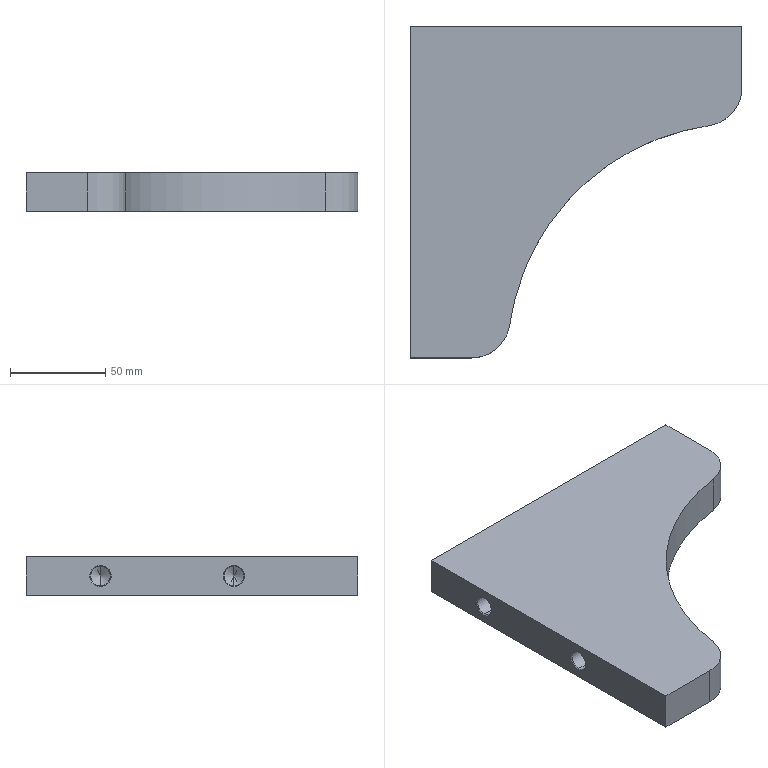Part | STEP file | Chain press plate | 1 solid | 21 faces | box 174 x 174 x 20 mm | volume 359243 mm3 | cone 8 | cylinder 7 | plane 6 | commonest cylinder face diameters 10.2 x4 40 x2 246 x1
STEP:
#1=CARTESIAN_POINT('',(0.,0.,0.));
#2=DIRECTION('',(0.,0.,1.));
#3=DIRECTION('',(1.,0.,0.));
#4=AXIS2_PLACEMENT_3D('',#1,#2,#3);
#5=CARTESIAN_POINT('',(0.5,-39.,15.1));
#6=VERTEX_POINT('',#5);
#7=CARTESIAN_POINT('',(0.,-39.,15.6));
#8=VERTEX_POINT('',#7);
#9=CARTESIAN_POINT('',(0.5,-39.,15.1));
#10=DIRECTION('',(-0.7071,0.,0.7071));
#11=VECTOR('',#10,1.);
#12=LINE('',#9,#11);
#13=CARTESIAN_POINT('',(0.5,-39.,10.));
#14=DIRECTION('',(-1.,0.,0.));
#15=DIRECTION('',(0.,0.,1.));
#16=AXIS2_PLACEMENT_3D('',#13,#14,#15);
#17=CONICAL_SURFACE('',#16,5.1,0.7854);
#18=CARTESIAN_POINT('',(6.283,0.));
#19=DIRECTION('',(0.,1.));
#20=VECTOR('',#19,1.);
#21=LINE('',#18,#20);
#22=(GEOMETRIC_REPRESENTATION_CONTEXT(2)PARAMETRIC_REPRESENTATION_CONTEXT()REPRESENTATION_CONTEXT('',''));
#23=DEFINITIONAL_REPRESENTATION('',(#21),#22);
#24=PCURVE('',#17,#23);
#25=CARTESIAN_POINT('',(0.5,-39.,10.));
#26=DIRECTION('',(-1.,0.,0.));
#27=DIRECTION('',(0.,0.,1.));
#28=AXIS2_PLACEMENT_3D('',#25,#26,#27);
#29=CONICAL_SURFACE('',#28,5.1,0.7854);
#30=CARTESIAN_POINT('',(0.,0.));
#31=DIRECTION('',(0.,1.));
#32=VECTOR('',#31,1.);
#33=LINE('',#30,#32);
#34=(GEOMETRIC_REPRESENTATION_CONTEXT(2)PARAMETRIC_REPRESENTATION_CONTEXT()REPRESENTATION_CONTEXT('',''));
#35=DEFINITIONAL_REPRESENTATION('',(#33),#34);
#36=PCURVE('',#29,#35);
#37=SURFACE_CURVE('',#12,(#24,#36),.PCURVE_S1.);
#38=EDGE_CURVE('',#6,#8,#37,.T.);
#39=ORIENTED_EDGE('',*,*,#38,.T.);
#40=CARTESIAN_POINT('',(0.,-39.,4.4));
#41=VERTEX_POINT('',#40);
#42=CARTESIAN_POINT('',(0.,-39.,10.));
#43=DIRECTION('',(1.,0.,0.));
#44=DIRECTION('',(0.,1.,0.));
#45=AXIS2_PLACEMENT_3D('',#42,#43,#44);
#46=CIRCLE('',#45,5.6);
#47=CARTESIAN_POINT('',(7.854,0.5));
#48=DIRECTION('',(-1.,0.));
#49=VECTOR('',#48,1.);
#50=LINE('',#47,#49);
#51=(GEOMETRIC_REPRESENTATION_CONTEXT(2)PARAMETRIC_REPRESENTATION_CONTEXT()REPRESENTATION_CONTEXT('',''));
#52=DEFINITIONAL_REPRESENTATION('',(#50),#51);
#53=PCURVE('',#17,#52);
#54=CARTESIAN_POINT('',(0.,0.,20.));
#55=DIRECTION('',(1.,0.,0.));
#56=DIRECTION('',(0.,1.,0.));
#57=AXIS2_PLACEMENT_3D('',#54,#55,#56);
#58=PLANE('',#57);
#59=CARTESIAN_POINT('',(-39.,-10.));
#60=DIRECTION('',(1.,0.));
#61=AXIS2_PLACEMENT_2D('',#59,#60);
#62=CIRCLE('',#61,5.6);
#63=(GEOMETRIC_REPRESENTATION_CONTEXT(2)PARAMETRIC_REPRESENTATION_CONTEXT()REPRESENTATION_CONTEXT('',''));
#64=DEFINITIONAL_REPRESENTATION('',(#62),#63);
#65=PCURVE('',#58,#64);
#66=SURFACE_CURVE('',#46,(#53,#65),.PCURVE_S1.);
#67=EDGE_CURVE('',#8,#41,#66,.T.);
#68=ORIENTED_EDGE('',*,*,#67,.T.);
#69=CARTESIAN_POINT('',(0.5,-39.,4.9));
#70=VERTEX_POINT('',#69);
#71=CARTESIAN_POINT('',(0.5,-39.,4.9));
#72=DIRECTION('',(-0.7071,0.,-0.7071));
#73=VECTOR('',#72,1.);
#74=LINE('',#71,#73);
#75=CARTESIAN_POINT('',(3.142,0.));
#76=DIRECTION('',(0.,1.));
#77=VECTOR('',#76,1.);
#78=LINE('',#75,#77);
#79=(GEOMETRIC_REPRESENTATION_CONTEXT(2)PARAMETRIC_REPRESENTATION_CONTEXT()REPRESENTATION_CONTEXT('',''));
#80=DEFINITIONAL_REPRESENTATION('',(#78),#79);
#81=PCURVE('',#17,#80);
#82=CARTESIAN_POINT('',(3.142,0.));
#83=DIRECTION('',(0.,1.));
#84=VECTOR('',#83,1.);
#85=LINE('',#82,#84);
#86=(GEOMETRIC_REPRESENTATION_CONTEXT(2)PARAMETRIC_REPRESENTATION_CONTEXT()REPRESENTATION_CONTEXT('',''));
#87=DEFINITIONAL_REPRESENTATION('',(#85),#86);
#88=PCURVE('',#29,#87);
#89=SURFACE_CURVE('',#74,(#81,#88),.PCURVE_S1.);
#90=EDGE_CURVE('',#70,#41,#89,.T.);
#91=ORIENTED_EDGE('',*,*,#90,.F.);
#92=CARTESIAN_POINT('',(0.5,-39.,10.));
#93=DIRECTION('',(-1.,0.,0.));
#94=DIRECTION('',(0.,0.,-1.));
#95=AXIS2_PLACEMENT_3D('',#92,#93,#94);
#96=CIRCLE('',#95,5.1);
#97=CARTESIAN_POINT('',(3.142,0.));
#98=DIRECTION('',(1.,0.));
#99=VECTOR('',#98,1.);
#100=LINE('',#97,#99);
#101=(GEOMETRIC_REPRESENTATION_CONTEXT(2)PARAMETRIC_REPRESENTATION_CONTEXT()REPRESENTATION_CONTEXT('',''));
#102=DEFINITIONAL_REPRESENTATION('',(#100),#101);
#103=PCURVE('',#17,#102);
#104=CARTESIAN_POINT('',(0.,-39.,10.));
#105=DIRECTION('',(-1.,0.,0.));
#106=DIRECTION('',(0.,0.,1.));
#107=AXIS2_PLACEMENT_3D('',#104,#105,#106);
#108=CYLINDRICAL_SURFACE('',#107,5.1);
#109=CARTESIAN_POINT('',(3.142,-0.5));
#110=DIRECTION('',(1.,0.));
#111=VECTOR('',#110,1.);
#112=LINE('',#109,#111);
#113=(GEOMETRIC_REPRESENTATION_CONTEXT(2)PARAMETRIC_REPRESENTATION_CONTEXT()REPRESENTATION_CONTEXT('',''));
#114=DEFINITIONAL_REPRESENTATION('',(#112),#113);
#115=PCURVE('',#108,#114);
#116=SURFACE_CURVE('',#96,(#103,#115),.PCURVE_S1.);
#117=EDGE_CURVE('',#70,#6,#116,.T.);
#118=ORIENTED_EDGE('',*,*,#117,.T.);
#119=EDGE_LOOP('',(#39,#68,#91,#118));
#120=FACE_BOUND('',#119,.F.);
#121=ADVANCED_FACE('',(#120),#17,.F.);
#122=CARTESIAN_POINT('',(0.5,-109.,15.1));
#123=VERTEX_POINT('',#122);
#124=CARTESIAN_POINT('',(0.,-109.,15.6));
#125=VERTEX_POINT('',#124);
#126=CARTESIAN_POINT('',(0.5,-109.,15.1));
#127=DIRECTION('',(-0.7071,0.,0.7071));
#128=VECTOR('',#127,1.);
#129=LINE('',#126,#128);
#130=CARTESIAN_POINT('',(0.5,-109.,10.));
#131=DIRECTION('',(-1.,0.,0.));
#132=DIRECTION('',(0.,0.,1.));
#133=AXIS2_PLACEMENT_3D('',#130,#131,#132);
#134=CONICAL_SURFACE('',#133,5.1,0.7854);
#135=CARTESIAN_POINT('',(6.283,0.));
#136=DIRECTION('',(0.,1.));
#137=VECTOR('',#136,1.);
#138=LINE('',#135,#137);
#139=(GEOMETRIC_REPRESENTATION_CONTEXT(2)PARAMETRIC_REPRESENTATION_CONTEXT()REPRESENTATION_CONTEXT('',''));
#140=DEFINITIONAL_REPRESENTATION('',(#138),#139);
#141=PCURVE('',#134,#140);
#142=CARTESIAN_POINT('',(0.5,-109.,10.));
#143=DIRECTION('',(-1.,0.,0.));
#144=DIRECTION('',(0.,0.,1.));
#145=AXIS2_PLACEMENT_3D('',#142,#143,#144);
#146=CONICAL_SURFACE('',#145,5.1,0.7854);
#147=CARTESIAN_POINT('',(0.,0.));
#148=DIRECTION('',(0.,1.));
#149=VECTOR('',#148,1.);
#150=LINE('',#147,#149);
#151=(GEOMETRIC_REPRESENTATION_CONTEXT(2)PARAMETRIC_REPRESENTATION_CONTEXT()REPRESENTATION_CONTEXT('',''));
#152=DEFINITIONAL_REPRESENTATION('',(#150),#151);
#153=PCURVE('',#146,#152);
#154=SURFACE_CURVE('',#129,(#141,#153),.PCURVE_S1.);
#155=EDGE_CURVE('',#123,#125,#154,.T.);
#156=ORIENTED_EDGE('',*,*,#155,.T.);
#157=CARTESIAN_POINT('',(0.,-109.,4.4));
#158=VERTEX_POINT('',#157);
#159=CARTESIAN_POINT('',(0.,-109.,10.));
#160=DIRECTION('',(1.,0.,0.));
#161=DIRECTION('',(0.,1.,0.));
#162=AXIS2_PLACEMENT_3D('',#159,#160,#161);
#163=CIRCLE('',#162,5.6);
#164=CARTESIAN_POINT('',(7.854,0.5));
#165=DIRECTION('',(-1.,0.));
#166=VECTOR('',#165,1.);
#167=LINE('',#164,#166);
#168=(GEOMETRIC_REPRESENTATION_CONTEXT(2)PARAMETRIC_REPRESENTATION_CONTEXT()REPRESENTATION_CONTEXT('',''));
#169=DEFINITIONAL_REPRESENTATION('',(#167),#168);
#170=PCURVE('',#134,#169);
#171=CARTESIAN_POINT('',(-109.,-10.));
#172=DIRECTION('',(1.,0.));
#173=AXIS2_PLACEMENT_2D('',#171,#172);
#174=CIRCLE('',#173,5.6);
#175=(GEOMETRIC_REPRESENTATION_CONTEXT(2)PARAMETRIC_REPRESENTATION_CONTEXT()REPRESENTATION_CONTEXT('',''));
#176=DEFINITIONAL_REPRESENTATION('',(#174),#175);
#177=PCURVE('',#58,#176);
#178=SURFACE_CURVE('',#163,(#170,#177),.PCURVE_S1.);
#179=EDGE_CURVE('',#125,#158,#178,.T.);
#180=ORIENTED_EDGE('',*,*,#179,.T.);
#181=CARTESIAN_POINT('',(0.5,-109.,4.9));
#182=VERTEX_POINT('',#181);
#183=CARTESIAN_POINT('',(0.5,-109.,4.9));
#184=DIRECTION('',(-0.7071,0.,-0.7071));
#185=VECTOR('',#184,1.);
#186=LINE('',#183,#185);
#187=CARTESIAN_POINT('',(3.142,0.));
#188=DIRECTION('',(0.,1.));
#189=VECTOR('',#188,1.);
#190=LINE('',#187,#189);
#191=(GEOMETRIC_REPRESENTATION_CONTEXT(2)PARAMETRIC_REPRESENTATION_CONTEXT()REPRESENTATION_CONTEXT('',''));
#192=DEFINITIONAL_REPRESENTATION('',(#190),#191);
#193=PCURVE('',#134,#192);
#194=CARTESIAN_POINT('',(3.142,0.));
#195=DIRECTION('',(0.,1.));
#196=VECTOR('',#195,1.);
#197=LINE('',#194,#196);
#198=(GEOMETRIC_REPRESENTATION_CONTEXT(2)PARAMETRIC_REPRESENTATION_CONTEXT()REPRESENTATION_CONTEXT('',''));
#199=DEFINITIONAL_REPRESENTATION('',(#197),#198);
#200=PCURVE('',#146,#199);
#201=SURFACE_CURVE('',#186,(#193,#200),.PCURVE_S1.);
#202=EDGE_CURVE('',#182,#158,#201,.T.);
#203=ORIENTED_EDGE('',*,*,#202,.F.);
#204=CARTESIAN_POINT('',(0.5,-109.,10.));
#205=DIRECTION('',(-1.,0.,0.));
#206=DIRECTION('',(0.,0.,-1.));
#207=AXIS2_PLACEMENT_3D('',#204,#205,#206);
#208=CIRCLE('',#207,5.1);
#209=CARTESIAN_POINT('',(3.142,0.));
#210=DIRECTION('',(1.,0.));
#211=VECTOR('',#210,1.);
#212=LINE('',#209,#211);
#213=(GEOMETRIC_REPRESENTATION_CONTEXT(2)PARAMETRIC_REPRESENTATION_CONTEXT()REPRESENTATION_CONTEXT('',''));
#214=DEFINITIONAL_REPRESENTATION('',(#212),#213);
#215=PCURVE('',#134,#214);
#216=CARTESIAN_POINT('',(0.,-109.,10.));
#217=DIRECTION('',(-1.,0.,0.));
#218=DIRECTION('',(0.,0.,1.));
#219=AXIS2_PLACEMENT_3D('',#216,#217,#218);
#220=CYLINDRICAL_SURFACE('',#219,5.1);
#221=CARTESIAN_POINT('',(3.142,-0.5));
#222=DIRECTION('',(1.,0.));
#223=VECTOR('',#222,1.);
#224=LINE('',#221,#223);
#225=(GEOMETRIC_REPRESENTATION_CONTEXT(2)PARAMETRIC_REPRESENTATION_CONTEXT()REPRESENTATION_CONTEXT('',''));
#226=DEFINITIONAL_REPRESENTATION('',(#224),#225);
#227=PCURVE('',#220,#226);
#228=SURFACE_CURVE('',#208,(#215,#227),.PCURVE_S1.);
#229=EDGE_CURVE('',#182,#123,#228,.T.);
#230=ORIENTED_EDGE('',*,*,#229,.T.);
#231=EDGE_LOOP('',(#156,#180,#203,#230));
#232=FACE_BOUND('',#231,.F.);
#233=ADVANCED_FACE('',(#232),#134,.F.);
#234=CARTESIAN_POINT('',(35.,-39.,15.1));
#235=VERTEX_POINT('',#234);
#236=CARTESIAN_POINT('',(0.,-39.,15.1));
#237=DIRECTION('',(-1.,0.,0.));
#238=VECTOR('',#237,1.);
#239=LINE('',#236,#238);
#240=CARTESIAN_POINT('',(6.283,0.));
#241=DIRECTION('',(0.,1.));
#242=VECTOR('',#241,1.);
#243=LINE('',#240,#242);
#244=(GEOMETRIC_REPRESENTATION_CONTEXT(2)PARAMETRIC_REPRESENTATION_CONTEXT()REPRESENTATION_CONTEXT('',''));
#245=DEFINITIONAL_REPRESENTATION('',(#243),#244);
#246=PCURVE('',#108,#245);
#247=CARTESIAN_POINT('',(0.,-39.,10.));
#248=DIRECTION('',(-1.,0.,0.));
#249=DIRECTION('',(0.,0.,1.));
#250=AXIS2_PLACEMENT_3D('',#247,#248,#249);
#251=CYLINDRICAL_SURFACE('',#250,5.1);
#252=CARTESIAN_POINT('',(0.,0.));
#253=DIRECTION('',(0.,1.));
#254=VECTOR('',#253,1.);
#255=LINE('',#252,#254);
#256=(GEOMETRIC_REPRESENTATION_CONTEXT(2)PARAMETRIC_REPRESENTATION_CONTEXT()REPRESENTATION_CONTEXT('',''));
#257=DEFINITIONAL_REPRESENTATION('',(#255),#256);
#258=PCURVE('',#251,#257);
#259=SURFACE_CURVE('',#239,(#246,#258),.PCURVE_S1.);
#260=EDGE_CURVE('',#235,#6,#259,.T.);
#261=ORIENTED_EDGE('',*,*,#260,.T.);
#262=ORIENTED_EDGE('',*,*,#117,.F.);
#263=CARTESIAN_POINT('',(35.,-39.,4.9));
#264=VERTEX_POINT('',#263);
#265=CARTESIAN_POINT('',(0.,-39.,4.9));
#266=DIRECTION('',(-1.,0.,0.));
#267=VECTOR('',#266,1.);
#268=LINE('',#265,#267);
#269=CARTESIAN_POINT('',(3.142,0.));
#270=DIRECTION('',(0.,1.));
#271=VECTOR('',#270,1.);
#272=LINE('',#269,#271);
#273=(GEOMETRIC_REPRESENTATION_CONTEXT(2)PARAMETRIC_REPRESENTATION_CONTEXT()REPRESENTATION_CONTEXT('',''));
#274=DEFINITIONAL_REPRESENTATION('',(#272),#273);
#275=PCURVE('',#108,#274);
#276=CARTESIAN_POINT('',(3.142,0.));
#277=DIRECTION('',(0.,1.));
#278=VECTOR('',#277,1.);
#279=LINE('',#276,#278);
#280=(GEOMETRIC_REPRESENTATION_CONTEXT(2)PARAMETRIC_REPRESENTATION_CONTEXT()REPRESENTATION_CONTEXT('',''));
#281=DEFINITIONAL_REPRESENTATION('',(#279),#280);
#282=PCURVE('',#251,#281);
#283=SURFACE_CURVE('',#268,(#275,#282),.PCURVE_S1.);
#284=EDGE_CURVE('',#264,#70,#283,.T.);
#285=ORIENTED_EDGE('',*,*,#284,.F.);
#286=CARTESIAN_POINT('',(35.,-39.,10.));
#287=DIRECTION('',(-1.,0.,0.));
#288=DIRECTION('',(0.,0.,1.));
#289=AXIS2_PLACEMENT_3D('',#286,#287,#288);
#290=CIRCLE('',#289,5.1);
#291=CARTESIAN_POINT('',(0.,-35.));
#292=DIRECTION('',(1.,0.));
#293=VECTOR('',#292,1.);
#294=LINE('',#291,#293);
#295=(GEOMETRIC_REPRESENTATION_CONTEXT(2)PARAMETRIC_REPRESENTATION_CONTEXT()REPRESENTATION_CONTEXT('',''));
#296=DEFINITIONAL_REPRESENTATION('',(#294),#295);
#297=PCURVE('',#108,#296);
#298=CARTESIAN_POINT('',(35.,-39.,10.));
#299=DIRECTION('',(-1.,0.,0.));
#300=DIRECTION('',(0.,0.,1.));
#301=AXIS2_PLACEMENT_3D('',#298,#299,#300);
#302=CONICAL_SURFACE('',#301,5.1,1.03);
#303=CARTESIAN_POINT('',(0.,0.));
#304=DIRECTION('',(1.,0.));
#305=VECTOR('',#304,1.);
#306=LINE('',#303,#305);
#307=(GEOMETRIC_REPRESENTATION_CONTEXT(2)PARAMETRIC_REPRESENTATION_CONTEXT()REPRESENTATION_CONTEXT('',''));
#308=DEFINITIONAL_REPRESENTATION('',(#306),#307);
#309=PCURVE('',#302,#308);
#310=SURFACE_CURVE('',#290,(#297,#309),.PCURVE_S1.);
#311=EDGE_CURVE('',#264,#235,#310,.T.);
#312=ORIENTED_EDGE('',*,*,#311,.T.);
#313=EDGE_LOOP('',(#261,#262,#285,#312));
#314=FACE_BOUND('',#313,.F.);
#315=ADVANCED_FACE('',(#314),#108,.F.);
#316=ORIENTED_EDGE('',*,*,#311,.F.);
#317=CARTESIAN_POINT('',(38.064,-39.,10.));
#318=VERTEX_POINT('',#317);
#319=CARTESIAN_POINT('',(35.,-39.,4.9));
#320=DIRECTION('',(-0.515,0.,-0.8572));
#321=VECTOR('',#320,1.);
#322=LINE('',#319,#321);
#323=CARTESIAN_POINT('',(3.142,-3.064));
#324=CARTESIAN_POINT('',(3.142,-3.018));
#325=CARTESIAN_POINT('',(3.142,-2.925));
#326=CARTESIAN_POINT('',(3.142,-2.786));
#327=CARTESIAN_POINT('',(3.142,-2.647));
#328=CARTESIAN_POINT('',(3.142,-2.507));
#329=CARTESIAN_POINT('',(3.142,-2.368));
#330=CARTESIAN_POINT('',(3.142,-2.229));
#331=CARTESIAN_POINT('',(3.142,-2.089));
#332=CARTESIAN_POINT('',(3.142,-1.95));
#333=CARTESIAN_POINT('',(3.142,-1.811));
#334=CARTESIAN_POINT('',(3.142,-1.671));
#335=CARTESIAN_POINT('',(3.142,-1.532));
#336=CARTESIAN_POINT('',(3.142,-1.393));
#337=CARTESIAN_POINT('',(3.142,-1.254));
#338=CARTESIAN_POINT('',(3.142,-1.114));
#339=CARTESIAN_POINT('',(3.142,-0.975));
#340=CARTESIAN_POINT('',(3.142,-0.8357));
#341=CARTESIAN_POINT('',(3.142,-0.6965));
#342=CARTESIAN_POINT('',(3.142,-0.5572));
#343=CARTESIAN_POINT('',(3.142,-0.4179));
#344=CARTESIAN_POINT('',(3.142,-0.2786));
#345=CARTESIAN_POINT('',(3.142,-0.1393));
#346=CARTESIAN_POINT('',(3.142,-0.04643));
#347=CARTESIAN_POINT('',(3.142,0.));
#348=B_SPLINE_CURVE_WITH_KNOTS('',3,(#323,#324,#325,#326,#327,#328,#329,#330,#331,#332,#333,#334,#335,#336,#337,#338,#339,#340,#341,#342,#343,#344,#345,#346,#347),.UNSPECIFIED.,.F.,.F.,(4,1,1,1,1,1,1,1,1,1,1,1,1,1,1,1,1,1,1,1,1,1,4),(-5.95,-5.679,-5.409,-5.138,-4.868,-4.598,-4.327,-4.057,-3.786,-3.516,-3.245,-2.975,-2.704,-2.434,-2.164,-1.893,-1.623,-1.352,-1.082,-0.8113,-0.5409,-0.2704,0.),.UNSPECIFIED.);
#349=(GEOMETRIC_REPRESENTATION_CONTEXT(2)PARAMETRIC_REPRESENTATION_CONTEXT()REPRESENTATION_CONTEXT('',''));
#350=DEFINITIONAL_REPRESENTATION('',(#348),#349);
#351=PCURVE('',#302,#350);
#352=CARTESIAN_POINT('',(35.,-39.,10.));
#353=DIRECTION('',(-1.,0.,0.));
#354=DIRECTION('',(0.,0.,1.));
#355=AXIS2_PLACEMENT_3D('',#352,#353,#354);
#356=CONICAL_SURFACE('',#355,5.1,1.03);
#357=CARTESIAN_POINT('',(3.142,-3.064));
#358=CARTESIAN_POINT('',(3.142,-3.018));
#359=CARTESIAN_POINT('',(3.142,-2.925));
#360=CARTESIAN_POINT('',(3.142,-2.786));
#361=CARTESIAN_POINT('',(3.142,-2.647));
#362=CARTESIAN_POINT('',(3.142,-2.507));
#363=CARTESIAN_POINT('',(3.142,-2.368));
#364=CARTESIAN_POINT('',(3.142,-2.229));
#365=CARTESIAN_POINT('',(3.142,-2.089));
#366=CARTESIAN_POINT('',(3.142,-1.95));
#367=CARTESIAN_POINT('',(3.142,-1.811));
#368=CARTESIAN_POINT('',(3.142,-1.671));
#369=CARTESIAN_POINT('',(3.142,-1.532));
#370=CARTESIAN_POINT('',(3.142,-1.393));
#371=CARTESIAN_POINT('',(3.142,-1.254));
#372=CARTESIAN_POINT('',(3.142,-1.114));
#373=CARTESIAN_POINT('',(3.142,-0.975));
#374=CARTESIAN_POINT('',(3.142,-0.8357));
#375=CARTESIAN_POINT('',(3.142,-0.6965));
#376=CARTESIAN_POINT('',(3.142,-0.5572));
#377=CARTESIAN_POINT('',(3.142,-0.4179));
#378=CARTESIAN_POINT('',(3.142,-0.2786));
#379=CARTESIAN_POINT('',(3.142,-0.1393));
#380=CARTESIAN_POINT('',(3.142,-0.04643));
#381=CARTESIAN_POINT('',(3.142,0.));
#382=B_SPLINE_CURVE_WITH_KNOTS('',3,(#357,#358,#359,#360,#361,#362,#363,#364,#365,#366,#367,#368,#369,#370,#371,#372,#373,#374,#375,#376,#377,#378,#379,#380,#381),.UNSPECIFIED.,.F.,.F.,(4,1,1,1,1,1,1,1,1,1,1,1,1,1,1,1,1,1,1,1,1,1,4),(-5.95,-5.679,-5.409,-5.138,-4.868,-4.598,-4.327,-4.057,-3.786,-3.516,-3.245,-2.975,-2.704,-2.434,-2.164,-1.893,-1.623,-1.352,-1.082,-0.8113,-0.5409,-0.2704,0.),.UNSPECIFIED.);
#383=(GEOMETRIC_REPRESENTATION_CONTEXT(2)PARAMETRIC_REPRESENTATION_CONTEXT()REPRESENTATION_CONTEXT('',''));
#384=DEFINITIONAL_REPRESENTATION('',(#382),#383);
#385=PCURVE('',#356,#384);
#386=SURFACE_CURVE('',#322,(#351,#385),.PCURVE_S1.);
#387=EDGE_CURVE('',#318,#264,#386,.T.);
#388=ORIENTED_EDGE('',*,*,#387,.F.);
#389=CARTESIAN_POINT('',(35.,-39.,15.1));
#390=DIRECTION('',(-0.515,0.,0.8572));
#391=VECTOR('',#390,1.);
#392=LINE('',#389,#391);
#393=CARTESIAN_POINT('',(6.283,0.));
#394=DIRECTION('',(0.,1.));
#395=VECTOR('',#394,1.);
#396=LINE('',#393,#395);
#397=(GEOMETRIC_REPRESENTATION_CONTEXT(2)PARAMETRIC_REPRESENTATION_CONTEXT()REPRESENTATION_CONTEXT('',''));
#398=DEFINITIONAL_REPRESENTATION('',(#396),#397);
#399=PCURVE('',#302,#398);
#400=CARTESIAN_POINT('',(0.,0.));
#401=DIRECTION('',(0.,1.));
#402=VECTOR('',#401,1.);
#403=LINE('',#400,#402);
#404=(GEOMETRIC_REPRESENTATION_CONTEXT(2)PARAMETRIC_REPRESENTATION_CONTEXT()REPRESENTATION_CONTEXT('',''));
#405=DEFINITIONAL_REPRESENTATION('',(#403),#404);
#406=PCURVE('',#356,#405);
#407=SURFACE_CURVE('',#392,(#399,#406),.PCURVE_S1.);
#408=EDGE_CURVE('',#318,#235,#407,.T.);
#409=ORIENTED_EDGE('',*,*,#408,.T.);
#410=EDGE_LOOP('',(#316,#388,#409));
#411=FACE_BOUND('',#410,.F.);
#412=ADVANCED_FACE('',(#411),#302,.F.);
#413=CARTESIAN_POINT('',(35.,-109.,15.1));
#414=VERTEX_POINT('',#413);
#415=CARTESIAN_POINT('',(0.,-109.,15.1));
#416=DIRECTION('',(-1.,0.,0.));
#417=VECTOR('',#416,1.);
#418=LINE('',#415,#417);
#419=CARTESIAN_POINT('',(6.283,0.));
#420=DIRECTION('',(0.,1.));
#421=VECTOR('',#420,1.);
#422=LINE('',#419,#421);
#423=(GEOMETRIC_REPRESENTATION_CONTEXT(2)PARAMETRIC_REPRESENTATION_CONTEXT()REPRESENTATION_CONTEXT('',''));
#424=DEFINITIONAL_REPRESENTATION('',(#422),#423);
#425=PCURVE('',#220,#424);
#426=CARTESIAN_POINT('',(0.,-109.,10.));
#427=DIRECTION('',(-1.,0.,0.));
#428=DIRECTION('',(0.,0.,1.));
#429=AXIS2_PLACEMENT_3D('',#426,#427,#428);
#430=CYLINDRICAL_SURFACE('',#429,5.1);
#431=CARTESIAN_POINT('',(0.,0.));
#432=DIRECTION('',(0.,1.));
#433=VECTOR('',#432,1.);
#434=LINE('',#431,#433);
#435=(GEOMETRIC_REPRESENTATION_CONTEXT(2)PARAMETRIC_REPRESENTATION_CONTEXT()REPRESENTATION_CONTEXT('',''));
#436=DEFINITIONAL_REPRESENTATION('',(#434),#435);
#437=PCURVE('',#430,#436);
#438=SURFACE_CURVE('',#418,(#425,#437),.PCURVE_S1.);
#439=EDGE_CURVE('',#414,#123,#438,.T.);
#440=ORIENTED_EDGE('',*,*,#439,.T.);
#441=ORIENTED_EDGE('',*,*,#229,.F.);
#442=CARTESIAN_POINT('',(35.,-109.,4.9));
#443=VERTEX_POINT('',#442);
#444=CARTESIAN_POINT('',(0.,-109.,4.9));
#445=DIRECTION('',(-1.,0.,0.));
#446=VECTOR('',#445,1.);
#447=LINE('',#444,#446);
#448=CARTESIAN_POINT('',(3.142,0.));
#449=DIRECTION('',(0.,1.));
#450=VECTOR('',#449,1.);
#451=LINE('',#448,#450);
#452=(GEOMETRIC_REPRESENTATION_CONTEXT(2)PARAMETRIC_REPRESENTATION_CONTEXT()REPRESENTATION_CONTEXT('',''));
#453=DEFINITIONAL_REPRESENTATION('',(#451),#452);
#454=PCURVE('',#220,#453);
#455=CARTESIAN_POINT('',(3.142,0.));
#456=DIRECTION('',(0.,1.));
#457=VECTOR('',#456,1.);
#458=LINE('',#455,#457);
#459=(GEOMETRIC_REPRESENTATION_CONTEXT(2)PARAMETRIC_REPRESENTATION_CONTEXT()REPRESENTATION_CONTEXT('',''));
#460=DEFINITIONAL_REPRESENTATION('',(#458),#459);
#461=PCURVE('',#430,#460);
#462=SURFACE_CURVE('',#447,(#454,#461),.PCURVE_S1.);
#463=EDGE_CURVE('',#443,#182,#462,.T.);
#464=ORIENTED_EDGE('',*,*,#463,.F.);
#465=CARTESIAN_POINT('',(35.,-109.,10.));
#466=DIRECTION('',(-1.,0.,0.));
#467=DIRECTION('',(0.,0.,1.));
#468=AXIS2_PLACEMENT_3D('',#465,#466,#467);
#469=CIRCLE('',#468,5.1);
#470=CARTESIAN_POINT('',(0.,-35.));
#471=DIRECTION('',(1.,0.));
#472=VECTOR('',#471,1.);
#473=LINE('',#470,#472);
#474=(GEOMETRIC_REPRESENTATION_CONTEXT(2)PARAMETRIC_REPRESENTATION_CONTEXT()REPRESENTATION_CONTEXT('',''));
#475=DEFINITIONAL_REPRESENTATION('',(#473),#474);
#476=PCURVE('',#220,#475);
#477=CARTESIAN_POINT('',(35.,-109.,10.));
#478=DIRECTION('',(-1.,0.,0.));
#479=DIRECTION('',(0.,0.,1.));
#480=AXIS2_PLACEMENT_3D('',#477,#478,#479);
#481=CONICAL_SURFACE('',#480,5.1,1.03);
#482=CARTESIAN_POINT('',(0.,0.));
#483=DIRECTION('',(1.,0.));
#484=VECTOR('',#483,1.);
#485=LINE('',#482,#484);
#486=(GEOMETRIC_REPRESENTATION_CONTEXT(2)PARAMETRIC_REPRESENTATION_CONTEXT()REPRESENTATION_CONTEXT('',''));
#487=DEFINITIONAL_REPRESENTATION('',(#485),#486);
#488=PCURVE('',#481,#487);
#489=SURFACE_CURVE('',#469,(#476,#488),.PCURVE_S1.);
#490=EDGE_CURVE('',#443,#414,#489,.T.);
#491=ORIENTED_EDGE('',*,*,#490,.T.);
#492=EDGE_LOOP('',(#440,#441,#464,#491));
#493=FACE_BOUND('',#492,.F.);
#494=ADVANCED_FACE('',(#493),#220,.F.);
#495=ORIENTED_EDGE('',*,*,#490,.F.);
#496=CARTESIAN_POINT('',(38.064,-109.,10.));
#497=VERTEX_POINT('',#496);
#498=CARTESIAN_POINT('',(35.,-109.,4.9));
#499=DIRECTION('',(-0.515,0.,-0.8572));
#500=VECTOR('',#499,1.);
#501=LINE('',#498,#500);
#502=CARTESIAN_POINT('',(3.142,0.));
#503=DIRECTION('',(0.,1.));
#504=VECTOR('',#503,1.);
#505=LINE('',#502,#504);
#506=(GEOMETRIC_REPRESENTATION_CONTEXT(2)PARAMETRIC_REPRESENTATION_CONTEXT()REPRESENTATION_CONTEXT('',''));
#507=DEFINITIONAL_REPRESENTATION('',(#505),#506);
#508=PCURVE('',#481,#507);
#509=CARTESIAN_POINT('',(35.,-109.,10.));
#510=DIRECTION('',(-1.,0.,0.));
#511=DIRECTION('',(0.,0.,1.));
#512=AXIS2_PLACEMENT_3D('',#509,#510,#511);
#513=CONICAL_SURFACE('',#512,5.1,1.03);
#514=CARTESIAN_POINT('',(3.142,0.));
#515=DIRECTION('',(0.,1.));
#516=VECTOR('',#515,1.);
#517=LINE('',#514,#516);
#518=(GEOMETRIC_REPRESENTATION_CONTEXT(2)PARAMETRIC_REPRESENTATION_CONTEXT()REPRESENTATION_CONTEXT('',''));
#519=DEFINITIONAL_REPRESENTATION('',(#517),#518);
#520=PCURVE('',#513,#519);
#521=SURFACE_CURVE('',#501,(#508,#520),.PCURVE_S1.);
#522=EDGE_CURVE('',#497,#443,#521,.T.);
#523=ORIENTED_EDGE('',*,*,#522,.F.);
#524=CARTESIAN_POINT('',(35.,-109.,15.1));
#525=DIRECTION('',(-0.515,0.,0.8572));
#526=VECTOR('',#525,1.);
#527=LINE('',#524,#526);
#528=CARTESIAN_POINT('',(6.283,0.));
#529=DIRECTION('',(0.,1.));
#530=VECTOR('',#529,1.);
#531=LINE('',#528,#530);
#532=(GEOMETRIC_REPRESENTATION_CONTEXT(2)PARAMETRIC_REPRESENTATION_CONTEXT()REPRESENTATION_CONTEXT('',''));
#533=DEFINITIONAL_REPRESENTATION('',(#531),#532);
#534=PCURVE('',#481,#533);
#535=CARTESIAN_POINT('',(0.,0.));
#536=DIRECTION('',(0.,1.));
#537=VECTOR('',#536,1.);
#538=LINE('',#535,#537);
#539=(GEOMETRIC_REPRESENTATION_CONTEXT(2)PARAMETRIC_REPRESENTATION_CONTEXT()REPRESENTATION_CONTEXT('',''));
#540=DEFINITIONAL_REPRESENTATION('',(#538),#539);
#541=PCURVE('',#513,#540);
#542=SURFACE_CURVE('',#527,(#534,#541),.PCURVE_S1.);
#543=EDGE_CURVE('',#497,#414,#542,.T.);
#544=ORIENTED_EDGE('',*,*,#543,.T.);
#545=EDGE_LOOP('',(#495,#523,#544));
#546=FACE_BOUND('',#545,.F.);
#547=ADVANCED_FACE('',(#546),#481,.F.);
#548=ORIENTED_EDGE('',*,*,#179,.T.);
#549=CARTESIAN_POINT('',(0.,-109.,10.));
#550=DIRECTION('',(1.,0.,0.));
#551=DIRECTION('',(0.,1.,0.));
#552=AXIS2_PLACEMENT_3D('',#549,#550,#551);
#553=CIRCLE('',#552,5.6);
#554=CARTESIAN_POINT('',(-109.,-10.));
#555=DIRECTION('',(1.,0.));
#556=AXIS2_PLACEMENT_2D('',#554,#555);
#557=CIRCLE('',#556,5.6);
#558=(GEOMETRIC_REPRESENTATION_CONTEXT(2)PARAMETRIC_REPRESENTATION_CONTEXT()REPRESENTATION_CONTEXT('',''));
#559=DEFINITIONAL_REPRESENTATION('',(#557),#558);
#560=PCURVE('',#58,#559);
#561=CARTESIAN_POINT('',(7.854,0.5));
#562=DIRECTION('',(-1.,0.));
#563=VECTOR('',#562,1.);
#564=LINE('',#561,#563);
#565=(GEOMETRIC_REPRESENTATION_CONTEXT(2)PARAMETRIC_REPRESENTATION_CONTEXT()REPRESENTATION_CONTEXT('',''));
#566=DEFINITIONAL_REPRESENTATION('',(#564),#565);
#567=PCURVE('',#146,#566);
#568=SURFACE_CURVE('',#553,(#560,#567),.PCURVE_S1.);
#569=EDGE_CURVE('',#158,#125,#568,.T.);
#570=ORIENTED_EDGE('',*,*,#569,.T.);
#571=EDGE_LOOP('',(#548,#570));
#572=FACE_BOUND('',#571,.T.);
#573=ORIENTED_EDGE('',*,*,#67,.T.);
#574=CARTESIAN_POINT('',(0.,-39.,10.));
#575=DIRECTION('',(1.,0.,0.));
#576=DIRECTION('',(0.,1.,0.));
#577=AXIS2_PLACEMENT_3D('',#574,#575,#576);
#578=CIRCLE('',#577,5.6);
#579=CARTESIAN_POINT('',(-39.,-10.));
#580=DIRECTION('',(1.,0.));
#581=AXIS2_PLACEMENT_2D('',#579,#580);
#582=CIRCLE('',#581,5.6);
#583=(GEOMETRIC_REPRESENTATION_CONTEXT(2)PARAMETRIC_REPRESENTATION_CONTEXT()REPRESENTATION_CONTEXT('',''));
#584=DEFINITIONAL_REPRESENTATION('',(#582),#583);
#585=PCURVE('',#58,#584);
#586=CARTESIAN_POINT('',(7.854,0.5));
#587=DIRECTION('',(-1.,0.));
#588=VECTOR('',#587,1.);
#589=LINE('',#586,#588);
#590=(GEOMETRIC_REPRESENTATION_CONTEXT(2)PARAMETRIC_REPRESENTATION_CONTEXT()REPRESENTATION_CONTEXT('',''));
#591=DEFINITIONAL_REPRESENTATION('',(#589),#590);
#592=PCURVE('',#29,#591);
#593=SURFACE_CURVE('',#578,(#585,#592),.PCURVE_S1.);
#594=EDGE_CURVE('',#41,#8,#593,.T.);
#595=ORIENTED_EDGE('',*,*,#594,.T.);
#596=EDGE_LOOP('',(#573,#595));
#597=FACE_BOUND('',#596,.T.);
#598=CARTESIAN_POINT('',(0.,0.,0.));
#599=VERTEX_POINT('',#598);
#600=CARTESIAN_POINT('',(0.,-174.,0.));
#601=VERTEX_POINT('',#600);
#602=CARTESIAN_POINT('',(0.,0.,0.));
#603=DIRECTION('',(0.,-1.,0.));
#604=VECTOR('',#603,1.);
#605=LINE('',#602,#604);
#606=CARTESIAN_POINT('',(0.,-20.));
#607=DIRECTION('',(-1.,0.));
#608=VECTOR('',#607,1.);
#609=LINE('',#606,#608);
#610=(GEOMETRIC_REPRESENTATION_CONTEXT(2)PARAMETRIC_REPRESENTATION_CONTEXT()REPRESENTATION_CONTEXT('',''));
#611=DEFINITIONAL_REPRESENTATION('',(#609),#610);
#612=PCURVE('',#58,#611);
#613=CARTESIAN_POINT('',(32.406,-154.,0.));
#614=DIRECTION('',(0.,0.,-1.));
#615=DIRECTION('',(-1.,0.,0.));
#616=AXIS2_PLACEMENT_3D('',#613,#614,#615);
#617=PLANE('',#616);
#618=CARTESIAN_POINT('',(32.406,154.));
#619=DIRECTION('',(0.,-1.));
#620=VECTOR('',#619,1.);
#621=LINE('',#618,#620);
#622=(GEOMETRIC_REPRESENTATION_CONTEXT(2)PARAMETRIC_REPRESENTATION_CONTEXT()REPRESENTATION_CONTEXT('',''));
#623=DEFINITIONAL_REPRESENTATION('',(#621),#622);
#624=PCURVE('',#617,#623);
#625=SURFACE_CURVE('',#605,(#612,#624),.PCURVE_S1.);
#626=EDGE_CURVE('',#599,#601,#625,.T.);
#627=ORIENTED_EDGE('',*,*,#626,.T.);
#628=CARTESIAN_POINT('',(0.,-174.,20.));
#629=VERTEX_POINT('',#628);
#630=CARTESIAN_POINT('',(0.,-174.,20.));
#631=DIRECTION('',(0.,0.,-1.));
#632=VECTOR('',#631,1.);
#633=LINE('',#630,#632);
#634=CARTESIAN_POINT('',(-174.,0.));
#635=DIRECTION('',(0.,-1.));
#636=VECTOR('',#635,1.);
#637=LINE('',#634,#636);
#638=(GEOMETRIC_REPRESENTATION_CONTEXT(2)PARAMETRIC_REPRESENTATION_CONTEXT()REPRESENTATION_CONTEXT('',''));
#639=DEFINITIONAL_REPRESENTATION('',(#637),#638);
#640=PCURVE('',#58,#639);
#641=CARTESIAN_POINT('',(32.406,-174.,20.));
#642=DIRECTION('',(0.,1.,0.));
#643=DIRECTION('',(0.,0.,1.));
#644=AXIS2_PLACEMENT_3D('',#641,#642,#643);
#645=PLANE('',#644);
#646=CARTESIAN_POINT('',(0.,-32.406));
#647=DIRECTION('',(-1.,0.));
#648=VECTOR('',#647,1.);
#649=LINE('',#646,#648);
#650=(GEOMETRIC_REPRESENTATION_CONTEXT(2)PARAMETRIC_REPRESENTATION_CONTEXT()REPRESENTATION_CONTEXT('',''));
#651=DEFINITIONAL_REPRESENTATION('',(#649),#650);
#652=PCURVE('',#645,#651);
#653=SURFACE_CURVE('',#633,(#640,#652),.PCURVE_S1.);
#654=EDGE_CURVE('',#629,#601,#653,.T.);
#655=ORIENTED_EDGE('',*,*,#654,.F.);
#656=CARTESIAN_POINT('',(0.,0.,20.));
#657=VERTEX_POINT('',#656);
#658=CARTESIAN_POINT('',(0.,0.,20.));
#659=DIRECTION('',(0.,-1.,0.));
#660=VECTOR('',#659,1.);
#661=LINE('',#658,#660);
#662=CARTESIAN_POINT('',(0.,0.));
#663=DIRECTION('',(-1.,0.));
#664=VECTOR('',#663,1.);
#665=LINE('',#662,#664);
#666=(GEOMETRIC_REPRESENTATION_CONTEXT(2)PARAMETRIC_REPRESENTATION_CONTEXT()REPRESENTATION_CONTEXT('',''));
#667=DEFINITIONAL_REPRESENTATION('',(#665),#666);
#668=PCURVE('',#58,#667);
#669=CARTESIAN_POINT('',(32.406,-154.,20.));
#670=DIRECTION('',(0.,0.,-1.));
#671=DIRECTION('',(-1.,0.,0.));
#672=AXIS2_PLACEMENT_3D('',#669,#670,#671);
#673=PLANE('',#672);
#674=CARTESIAN_POINT('',(32.406,154.));
#675=DIRECTION('',(0.,-1.));
#676=VECTOR('',#675,1.);
#677=LINE('',#674,#676);
#678=(GEOMETRIC_REPRESENTATION_CONTEXT(2)PARAMETRIC_REPRESENTATION_CONTEXT()REPRESENTATION_CONTEXT('',''));
#679=DEFINITIONAL_REPRESENTATION('',(#677),#678);
#680=PCURVE('',#673,#679);
#681=SURFACE_CURVE('',#661,(#668,#680),.PCURVE_S1.);
#682=EDGE_CURVE('',#657,#629,#681,.T.);
#683=ORIENTED_EDGE('',*,*,#682,.F.);
#684=CARTESIAN_POINT('',(0.,0.,20.));
#685=DIRECTION('',(0.,0.,-1.));
#686=VECTOR('',#685,1.);
#687=LINE('',#684,#686);
#688=CARTESIAN_POINT('',(0.,0.));
#689=DIRECTION('',(0.,-1.));
#690=VECTOR('',#689,1.);
#691=LINE('',#688,#690);
#692=(GEOMETRIC_REPRESENTATION_CONTEXT(2)PARAMETRIC_REPRESENTATION_CONTEXT()REPRESENTATION_CONTEXT('',''));
#693=DEFINITIONAL_REPRESENTATION('',(#691),#692);
#694=PCURVE('',#58,#693);
#695=CARTESIAN_POINT('',(0.,0.,20.));
#696=DIRECTION('',(0.,-1.,0.));
#697=DIRECTION('',(0.,0.,-1.));
#698=AXIS2_PLACEMENT_3D('',#695,#696,#697);
#699=PLANE('',#698);
#700=CARTESIAN_POINT('',(0.,0.));
#701=DIRECTION('',(1.,0.));
#702=VECTOR('',#701,1.);
#703=LINE('',#700,#702);
#704=(GEOMETRIC_REPRESENTATION_CONTEXT(2)PARAMETRIC_REPRESENTATION_CONTEXT()REPRESENTATION_CONTEXT('',''));
#705=DEFINITIONAL_REPRESENTATION('',(#703),#704);
#706=PCURVE('',#699,#705);
#707=SURFACE_CURVE('',#687,(#694,#706),.PCURVE_S1.);
#708=EDGE_CURVE('',#657,#599,#707,.T.);
#709=ORIENTED_EDGE('',*,*,#708,.T.);
#710=EDGE_LOOP('',(#627,#655,#683,#709));
#711=FACE_BOUND('',#710,.T.);
#712=ADVANCED_FACE('',(#572,#597,#711),#58,.F.);
#713=CARTESIAN_POINT('',(32.406,-174.,0.));
#714=VERTEX_POINT('',#713);
#715=CARTESIAN_POINT('',(32.406,-174.,0.));
#716=DIRECTION('',(1.,0.,0.));
#717=VECTOR('',#716,1.);
#718=LINE('',#715,#717);
#719=CARTESIAN_POINT('',(-20.,0.));
#720=DIRECTION('',(0.,1.));
#721=VECTOR('',#720,1.);
#722=LINE('',#719,#721);
#723=(GEOMETRIC_REPRESENTATION_CONTEXT(2)PARAMETRIC_REPRESENTATION_CONTEXT()REPRESENTATION_CONTEXT('',''));
#724=DEFINITIONAL_REPRESENTATION('',(#722),#723);
#725=PCURVE('',#645,#724);
#726=CARTESIAN_POINT('',(0.,-20.));
#727=DIRECTION('',(-1.,0.));
#728=VECTOR('',#727,1.);
#729=LINE('',#726,#728);
#730=(GEOMETRIC_REPRESENTATION_CONTEXT(2)PARAMETRIC_REPRESENTATION_CONTEXT()REPRESENTATION_CONTEXT('',''));
#731=DEFINITIONAL_REPRESENTATION('',(#729),#730);
#732=PCURVE('',#617,#731);
#733=SURFACE_CURVE('',#718,(#725,#732),.PCURVE_S1.);
#734=EDGE_CURVE('',#601,#714,#733,.T.);
#735=ORIENTED_EDGE('',*,*,#734,.T.);
#736=CARTESIAN_POINT('',(32.406,-174.,20.));
#737=VERTEX_POINT('',#736);
#738=CARTESIAN_POINT('',(32.406,-174.,20.));
#739=DIRECTION('',(0.,0.,-1.));
#740=VECTOR('',#739,1.);
#741=LINE('',#738,#740);
#742=CARTESIAN_POINT('',(0.,0.));
#743=DIRECTION('',(-1.,0.));
#744=VECTOR('',#743,1.);
#745=LINE('',#742,#744);
#746=(GEOMETRIC_REPRESENTATION_CONTEXT(2)PARAMETRIC_REPRESENTATION_CONTEXT()REPRESENTATION_CONTEXT('',''));
#747=DEFINITIONAL_REPRESENTATION('',(#745),#746);
#748=PCURVE('',#645,#747);
#749=CARTESIAN_POINT('',(32.406,-154.,20.));
#750=DIRECTION('',(0.,0.,-1.));
#751=DIRECTION('',(-1.,0.,0.));
#752=AXIS2_PLACEMENT_3D('',#749,#750,#751);
#753=CYLINDRICAL_SURFACE('',#752,20.);
#754=CARTESIAN_POINT('',(4.712,0.));
#755=DIRECTION('',(0.,1.));
#756=VECTOR('',#755,1.);
#757=LINE('',#754,#756);
#758=(GEOMETRIC_REPRESENTATION_CONTEXT(2)PARAMETRIC_REPRESENTATION_CONTEXT()REPRESENTATION_CONTEXT('',''));
#759=DEFINITIONAL_REPRESENTATION('',(#757),#758);
#760=PCURVE('',#753,#759);
#761=SURFACE_CURVE('',#741,(#748,#760),.PCURVE_S1.);
#762=EDGE_CURVE('',#737,#714,#761,.T.);
#763=ORIENTED_EDGE('',*,*,#762,.F.);
#764=CARTESIAN_POINT('',(32.406,-174.,20.));
#765=DIRECTION('',(1.,0.,0.));
#766=VECTOR('',#765,1.);
#767=LINE('',#764,#766);
#768=CARTESIAN_POINT('',(0.,0.));
#769=DIRECTION('',(0.,1.));
#770=VECTOR('',#769,1.);
#771=LINE('',#768,#770);
#772=(GEOMETRIC_REPRESENTATION_CONTEXT(2)PARAMETRIC_REPRESENTATION_CONTEXT()REPRESENTATION_CONTEXT('',''));
#773=DEFINITIONAL_REPRESENTATION('',(#771),#772);
#774=PCURVE('',#645,#773);
#775=CARTESIAN_POINT('',(0.,-20.));
#776=DIRECTION('',(-1.,0.));
#777=VECTOR('',#776,1.);
#778=LINE('',#775,#777);
#779=(GEOMETRIC_REPRESENTATION_CONTEXT(2)PARAMETRIC_REPRESENTATION_CONTEXT()REPRESENTATION_CONTEXT('',''));
#780=DEFINITIONAL_REPRESENTATION('',(#778),#779);
#781=PCURVE('',#673,#780);
#782=SURFACE_CURVE('',#767,(#774,#781),.PCURVE_S1.);
#783=EDGE_CURVE('',#629,#737,#782,.T.);
#784=ORIENTED_EDGE('',*,*,#783,.F.);
#785=ORIENTED_EDGE('',*,*,#654,.T.);
#786=EDGE_LOOP('',(#735,#763,#784,#785));
#787=FACE_BOUND('',#786,.T.);
#788=ADVANCED_FACE('',(#787),#645,.F.);
#789=CARTESIAN_POINT('',(52.209,-156.797,0.));
#790=VERTEX_POINT('',#789);
#791=CARTESIAN_POINT('',(32.406,-154.,0.));
#792=DIRECTION('',(0.,0.,1.));
#793=DIRECTION('',(-1.,0.,0.));
#794=AXIS2_PLACEMENT_3D('',#791,#792,#793);
#795=CIRCLE('',#794,20.);
#796=CARTESIAN_POINT('',(6.283,20.));
#797=DIRECTION('',(-1.,0.));
#798=VECTOR('',#797,1.);
#799=LINE('',#796,#798);
#800=(GEOMETRIC_REPRESENTATION_CONTEXT(2)PARAMETRIC_REPRESENTATION_CONTEXT()REPRESENTATION_CONTEXT('',''));
#801=DEFINITIONAL_REPRESENTATION('',(#799),#800);
#802=PCURVE('',#753,#801);
#803=CARTESIAN_POINT('',(20.,0.));
#804=CARTESIAN_POINT('',(20.,-34.641));
#805=CARTESIAN_POINT('',(-10.,-17.321));
#806=CARTESIAN_POINT('',(-40.,0.));
#807=CARTESIAN_POINT('',(-10.,17.321));
#808=CARTESIAN_POINT('',(20.,34.641));
#809=CARTESIAN_POINT('',(20.,0.));
#810=(BOUNDED_CURVE()B_SPLINE_CURVE(2,(#803,#804,#805,#806,#807,#808,#809),.UNSPECIFIED.,.T.,.F.)B_SPLINE_CURVE_WITH_KNOTS((1,2,2,2,2,1),(-2.094,0.,2.094,4.189,6.283,8.378),.UNSPECIFIED.)CURVE()GEOMETRIC_REPRESENTATION_ITEM()RATIONAL_B_SPLINE_CURVE((1.,0.5,1.,0.5,1.,0.5,1.))REPRESENTATION_ITEM(''));
#811=(GEOMETRIC_REPRESENTATION_CONTEXT(2)PARAMETRIC_REPRESENTATION_CONTEXT()REPRESENTATION_CONTEXT('',''));
#812=DEFINITIONAL_REPRESENTATION('',(#810),#811);
#813=PCURVE('',#617,#812);
#814=SURFACE_CURVE('',#795,(#802,#813),.PCURVE_S1.);
#815=EDGE_CURVE('',#714,#790,#814,.T.);
#816=ORIENTED_EDGE('',*,*,#815,.T.);
#817=CARTESIAN_POINT('',(52.209,-156.797,20.));
#818=VERTEX_POINT('',#817);
#819=CARTESIAN_POINT('',(52.209,-156.797,20.));
#820=DIRECTION('',(0.,0.,-1.));
#821=VECTOR('',#820,1.);
#822=LINE('',#819,#821);
#823=CARTESIAN_POINT('',(3.282,0.));
#824=DIRECTION('',(0.,1.));
#825=VECTOR('',#824,1.);
#826=LINE('',#823,#825);
#827=(GEOMETRIC_REPRESENTATION_CONTEXT(2)PARAMETRIC_REPRESENTATION_CONTEXT()REPRESENTATION_CONTEXT('',''));
#828=DEFINITIONAL_REPRESENTATION('',(#826),#827);
#829=PCURVE('',#753,#828);
#830=CARTESIAN_POINT('',(174.,-174.,20.));
#831=DIRECTION('',(0.,0.,-1.));
#832=DIRECTION('',(-1.,0.,0.));
#833=AXIS2_PLACEMENT_3D('',#830,#831,#832);
#834=CYLINDRICAL_SURFACE('',#833,123.);
#835=CARTESIAN_POINT('',(0.1403,0.));
#836=DIRECTION('',(0.,1.));
#837=VECTOR('',#836,1.);
#838=LINE('',#835,#837);
#839=(GEOMETRIC_REPRESENTATION_CONTEXT(2)PARAMETRIC_REPRESENTATION_CONTEXT()REPRESENTATION_CONTEXT('',''));
#840=DEFINITIONAL_REPRESENTATION('',(#838),#839);
#841=PCURVE('',#834,#840);
#842=SURFACE_CURVE('',#822,(#829,#841),.PCURVE_S1.);
#843=EDGE_CURVE('',#818,#790,#842,.T.);
#844=ORIENTED_EDGE('',*,*,#843,.F.);
#845=CARTESIAN_POINT('',(32.406,-154.,20.));
#846=DIRECTION('',(0.,0.,1.));
#847=DIRECTION('',(-1.,0.,0.));
#848=AXIS2_PLACEMENT_3D('',#845,#846,#847);
#849=CIRCLE('',#848,20.);
#850=CARTESIAN_POINT('',(6.283,0.));
#851=DIRECTION('',(-1.,0.));
#852=VECTOR('',#851,1.);
#853=LINE('',#850,#852);
#854=(GEOMETRIC_REPRESENTATION_CONTEXT(2)PARAMETRIC_REPRESENTATION_CONTEXT()REPRESENTATION_CONTEXT('',''));
#855=DEFINITIONAL_REPRESENTATION('',(#853),#854);
#856=PCURVE('',#753,#855);
#857=CARTESIAN_POINT('',(20.,0.));
#858=CARTESIAN_POINT('',(20.,-34.641));
#859=CARTESIAN_POINT('',(-10.,-17.321));
#860=CARTESIAN_POINT('',(-40.,0.));
#861=CARTESIAN_POINT('',(-10.,17.321));
#862=CARTESIAN_POINT('',(20.,34.641));
#863=CARTESIAN_POINT('',(20.,0.));
#864=(BOUNDED_CURVE()B_SPLINE_CURVE(2,(#857,#858,#859,#860,#861,#862,#863),.UNSPECIFIED.,.T.,.F.)B_SPLINE_CURVE_WITH_KNOTS((1,2,2,2,2,1),(-2.094,0.,2.094,4.189,6.283,8.378),.UNSPECIFIED.)CURVE()GEOMETRIC_REPRESENTATION_ITEM()RATIONAL_B_SPLINE_CURVE((1.,0.5,1.,0.5,1.,0.5,1.))REPRESENTATION_ITEM(''));
#865=(GEOMETRIC_REPRESENTATION_CONTEXT(2)PARAMETRIC_REPRESENTATION_CONTEXT()REPRESENTATION_CONTEXT('',''));
#866=DEFINITIONAL_REPRESENTATION('',(#864),#865);
#867=PCURVE('',#673,#866);
#868=SURFACE_CURVE('',#849,(#856,#867),.PCURVE_S1.);
#869=EDGE_CURVE('',#737,#818,#868,.T.);
#870=ORIENTED_EDGE('',*,*,#869,.F.);
#871=ORIENTED_EDGE('',*,*,#762,.T.);
#872=EDGE_LOOP('',(#816,#844,#870,#871));
#873=FACE_BOUND('',#872,.T.);
#874=ADVANCED_FACE('',(#873),#753,.T.);
#875=ORIENTED_EDGE('',*,*,#843,.F.);
#876=CARTESIAN_POINT('',(156.797,-52.209,20.));
#877=VERTEX_POINT('',#876);
#878=CARTESIAN_POINT('',(174.,-174.,20.));
#879=DIRECTION('',(0.,0.,-1.));
#880=DIRECTION('',(1.,0.,0.));
#881=AXIS2_PLACEMENT_3D('',#878,#879,#880);
#882=CIRCLE('',#881,123.);
#883=CARTESIAN_POINT('',(-3.142,0.));
#884=DIRECTION('',(1.,0.));
#885=VECTOR('',#884,1.);
#886=LINE('',#883,#885);
#887=(GEOMETRIC_REPRESENTATION_CONTEXT(2)PARAMETRIC_REPRESENTATION_CONTEXT()REPRESENTATION_CONTEXT('',''));
#888=DEFINITIONAL_REPRESENTATION('',(#886),#887);
#889=PCURVE('',#834,#888);
#890=CARTESIAN_POINT('',(-141.594,-20.));
#891=DIRECTION('',(-1.,0.));
#892=AXIS2_PLACEMENT_2D('',#890,#891);
#893=CIRCLE('',#892,123.);
#894=(GEOMETRIC_REPRESENTATION_CONTEXT(2)PARAMETRIC_REPRESENTATION_CONTEXT()REPRESENTATION_CONTEXT('',''));
#895=DEFINITIONAL_REPRESENTATION('',(#893),#894);
#896=PCURVE('',#673,#895);
#897=SURFACE_CURVE('',#882,(#889,#896),.PCURVE_S1.);
#898=EDGE_CURVE('',#818,#877,#897,.T.);
#899=ORIENTED_EDGE('',*,*,#898,.T.);
#900=CARTESIAN_POINT('',(156.797,-52.209,0.));
#901=VERTEX_POINT('',#900);
#902=CARTESIAN_POINT('',(156.797,-52.209,20.));
#903=DIRECTION('',(0.,0.,-1.));
#904=VECTOR('',#903,1.);
#905=LINE('',#902,#904);
#906=CARTESIAN_POINT('',(1.43,0.));
#907=DIRECTION('',(0.,1.));
#908=VECTOR('',#907,1.);
#909=LINE('',#906,#908);
#910=(GEOMETRIC_REPRESENTATION_CONTEXT(2)PARAMETRIC_REPRESENTATION_CONTEXT()REPRESENTATION_CONTEXT('',''));
#911=DEFINITIONAL_REPRESENTATION('',(#909),#910);
#912=PCURVE('',#834,#911);
#913=CARTESIAN_POINT('',(154.,-32.406,20.));
#914=DIRECTION('',(0.,0.,-1.));
#915=DIRECTION('',(-1.,0.,0.));
#916=AXIS2_PLACEMENT_3D('',#913,#914,#915);
#917=CYLINDRICAL_SURFACE('',#916,20.);
#918=CARTESIAN_POINT('',(4.572,0.));
#919=DIRECTION('',(0.,1.));
#920=VECTOR('',#919,1.);
#921=LINE('',#918,#920);
#922=(GEOMETRIC_REPRESENTATION_CONTEXT(2)PARAMETRIC_REPRESENTATION_CONTEXT()REPRESENTATION_CONTEXT('',''));
#923=DEFINITIONAL_REPRESENTATION('',(#921),#922);
#924=PCURVE('',#917,#923);
#925=SURFACE_CURVE('',#905,(#912,#924),.PCURVE_S1.);
#926=EDGE_CURVE('',#877,#901,#925,.T.);
#927=ORIENTED_EDGE('',*,*,#926,.T.);
#928=CARTESIAN_POINT('',(174.,-174.,0.));
#929=DIRECTION('',(0.,0.,-1.));
#930=DIRECTION('',(1.,0.,0.));
#931=AXIS2_PLACEMENT_3D('',#928,#929,#930);
#932=CIRCLE('',#931,123.);
#933=CARTESIAN_POINT('',(-3.142,20.));
#934=DIRECTION('',(1.,0.));
#935=VECTOR('',#934,1.);
#936=LINE('',#933,#935);
#937=(GEOMETRIC_REPRESENTATION_CONTEXT(2)PARAMETRIC_REPRESENTATION_CONTEXT()REPRESENTATION_CONTEXT('',''));
#938=DEFINITIONAL_REPRESENTATION('',(#936),#937);
#939=PCURVE('',#834,#938);
#940=CARTESIAN_POINT('',(-141.594,-20.));
#941=DIRECTION('',(-1.,0.));
#942=AXIS2_PLACEMENT_2D('',#940,#941);
#943=CIRCLE('',#942,123.);
#944=(GEOMETRIC_REPRESENTATION_CONTEXT(2)PARAMETRIC_REPRESENTATION_CONTEXT()REPRESENTATION_CONTEXT('',''));
#945=DEFINITIONAL_REPRESENTATION('',(#943),#944);
#946=PCURVE('',#617,#945);
#947=SURFACE_CURVE('',#932,(#939,#946),.PCURVE_S1.);
#948=EDGE_CURVE('',#790,#901,#947,.T.);
#949=ORIENTED_EDGE('',*,*,#948,.F.);
#950=EDGE_LOOP('',(#875,#899,#927,#949));
#951=FACE_BOUND('',#950,.F.);
#952=ADVANCED_FACE('',(#951),#834,.F.);
#953=CARTESIAN_POINT('',(174.,-32.406,0.));
#954=VERTEX_POINT('',#953);
#955=CARTESIAN_POINT('',(154.,-32.406,0.));
#956=DIRECTION('',(0.,0.,1.));
#957=DIRECTION('',(-1.,0.,0.));
#958=AXIS2_PLACEMENT_3D('',#955,#956,#957);
#959=CIRCLE('',#958,20.);
#960=CARTESIAN_POINT('',(6.283,20.));
#961=DIRECTION('',(-1.,0.));
#962=VECTOR('',#961,1.);
#963=LINE('',#960,#962);
#964=(GEOMETRIC_REPRESENTATION_CONTEXT(2)PARAMETRIC_REPRESENTATION_CONTEXT()REPRESENTATION_CONTEXT('',''));
#965=DEFINITIONAL_REPRESENTATION('',(#963),#964);
#966=PCURVE('',#917,#965);
#967=CARTESIAN_POINT('',(-101.594,121.594));
#968=CARTESIAN_POINT('',(-101.594,86.953));
#969=CARTESIAN_POINT('',(-131.594,104.274));
#970=CARTESIAN_POINT('',(-161.594,121.594));
#971=CARTESIAN_POINT('',(-131.594,138.915));
#972=CARTESIAN_POINT('',(-101.594,156.236));
#973=CARTESIAN_POINT('',(-101.594,121.594));
#974=(BOUNDED_CURVE()B_SPLINE_CURVE(2,(#967,#968,#969,#970,#971,#972,#973),.UNSPECIFIED.,.T.,.F.)B_SPLINE_CURVE_WITH_KNOTS((1,2,2,2,2,1),(-2.094,0.,2.094,4.189,6.283,8.378),.UNSPECIFIED.)CURVE()GEOMETRIC_REPRESENTATION_ITEM()RATIONAL_B_SPLINE_CURVE((1.,0.5,1.,0.5,1.,0.5,1.))REPRESENTATION_ITEM(''));
#975=(GEOMETRIC_REPRESENTATION_CONTEXT(2)PARAMETRIC_REPRESENTATION_CONTEXT()REPRESENTATION_CONTEXT('',''));
#976=DEFINITIONAL_REPRESENTATION('',(#974),#975);
#977=PCURVE('',#617,#976);
#978=SURFACE_CURVE('',#959,(#966,#977),.PCURVE_S1.);
#979=EDGE_CURVE('',#901,#954,#978,.T.);
#980=ORIENTED_EDGE('',*,*,#979,.T.);
#981=CARTESIAN_POINT('',(174.,-32.406,20.));
#982=VERTEX_POINT('',#981);
#983=CARTESIAN_POINT('',(174.,-32.406,20.));
#984=DIRECTION('',(0.,0.,-1.));
#985=VECTOR('',#984,1.);
#986=LINE('',#983,#985);
#987=CARTESIAN_POINT('',(3.142,0.));
#988=DIRECTION('',(0.,1.));
#989=VECTOR('',#988,1.);
#990=LINE('',#987,#989);
#991=(GEOMETRIC_REPRESENTATION_CONTEXT(2)PARAMETRIC_REPRESENTATION_CONTEXT()REPRESENTATION_CONTEXT('',''));
#992=DEFINITIONAL_REPRESENTATION('',(#990),#991);
#993=PCURVE('',#917,#992);
#994=CARTESIAN_POINT('',(174.,0.,20.));
#995=DIRECTION('',(-1.,0.,0.));
#996=DIRECTION('',(0.,0.,1.));
#997=AXIS2_PLACEMENT_3D('',#994,#995,#996);
#998=PLANE('',#997);
#999=CARTESIAN_POINT('',(0.,-32.406));
#1000=DIRECTION('',(-1.,0.));
#1001=VECTOR('',#1000,1.);
#1002=LINE('',#999,#1001);
#1003=(GEOMETRIC_REPRESENTATION_CONTEXT(2)PARAMETRIC_REPRESENTATION_CONTEXT()REPRESENTATION_CONTEXT('',''));
#1004=DEFINITIONAL_REPRESENTATION('',(#1002),#1003);
#1005=PCURVE('',#998,#1004);
#1006=SURFACE_CURVE('',#986,(#993,#1005),.PCURVE_S1.);
#1007=EDGE_CURVE('',#982,#954,#1006,.T.);
#1008=ORIENTED_EDGE('',*,*,#1007,.F.);
#1009=CARTESIAN_POINT('',(154.,-32.406,20.));
#1010=DIRECTION('',(0.,0.,1.));
#1011=DIRECTION('',(-1.,0.,0.));
#1012=AXIS2_PLACEMENT_3D('',#1009,#1010,#1011);
#1013=CIRCLE('',#1012,20.);
#1014=CARTESIAN_POINT('',(6.283,0.));
#1015=DIRECTION('',(-1.,0.));
#1016=VECTOR('',#1015,1.);
#1017=LINE('',#1014,#1016);
#1018=(GEOMETRIC_REPRESENTATION_CONTEXT(2)PARAMETRIC_REPRESENTATION_CONTEXT()REPRESENTATION_CONTEXT('',''));
#1019=DEFINITIONAL_REPRESENTATION('',(#1017),#1018);
#1020=PCURVE('',#917,#1019);
#1021=CARTESIAN_POINT('',(-101.594,121.594));
#1022=CARTESIAN_POINT('',(-101.594,86.953));
#1023=CARTESIAN_POINT('',(-131.594,104.274));
#1024=CARTESIAN_POINT('',(-161.594,121.594));
#1025=CARTESIAN_POINT('',(-131.594,138.915));
#1026=CARTESIAN_POINT('',(-101.594,156.236));
#1027=CARTESIAN_POINT('',(-101.594,121.594));
#1028=(BOUNDED_CURVE()B_SPLINE_CURVE(2,(#1021,#1022,#1023,#1024,#1025,#1026,#1027),.UNSPECIFIED.,.T.,.F.)B_SPLINE_CURVE_WITH_KNOTS((1,2,2,2,2,1),(-2.094,0.,2.094,4.189,6.283,8.378),.UNSPECIFIED.)CURVE()GEOMETRIC_REPRESENTATION_ITEM()RATIONAL_B_SPLINE_CURVE((1.,0.5,1.,0.5,1.,0.5,1.))REPRESENTATION_ITEM(''));
#1029=(GEOMETRIC_REPRESENTATION_CONTEXT(2)PARAMETRIC_REPRESENTATION_CONTEXT()REPRESENTATION_CONTEXT('',''));
#1030=DEFINITIONAL_REPRESENTATION('',(#1028),#1029);
#1031=PCURVE('',#673,#1030);
#1032=SURFACE_CURVE('',#1013,(#1020,#1031),.PCURVE_S1.);
#1033=EDGE_CURVE('',#877,#982,#1032,.T.);
#1034=ORIENTED_EDGE('',*,*,#1033,.F.);
#1035=ORIENTED_EDGE('',*,*,#926,.T.);
#1036=EDGE_LOOP('',(#980,#1008,#1034,#1035));
#1037=FACE_BOUND('',#1036,.T.);
#1038=ADVANCED_FACE('',(#1037),#917,.T.);
#1039=CARTESIAN_POINT('',(174.,0.,0.));
#1040=VERTEX_POINT('',#1039);
#1041=CARTESIAN_POINT('',(174.,0.,0.));
#1042=DIRECTION('',(0.,1.,0.));
#1043=VECTOR('',#1042,1.);
#1044=LINE('',#1041,#1043);
#1045=CARTESIAN_POINT('',(-20.,0.));
#1046=DIRECTION('',(0.,1.));
#1047=VECTOR('',#1046,1.);
#1048=LINE('',#1045,#1047);
#1049=(GEOMETRIC_REPRESENTATION_CONTEXT(2)PARAMETRIC_REPRESENTATION_CONTEXT()REPRESENTATION_CONTEXT('',''));
#1050=DEFINITIONAL_REPRESENTATION('',(#1048),#1049);
#1051=PCURVE('',#998,#1050);
#1052=CARTESIAN_POINT('',(-141.594,154.));
#1053=DIRECTION('',(0.,1.));
#1054=VECTOR('',#1053,1.);
#1055=LINE('',#1052,#1054);
#1056=(GEOMETRIC_REPRESENTATION_CONTEXT(2)PARAMETRIC_REPRESENTATION_CONTEXT()REPRESENTATION_CONTEXT('',''));
#1057=DEFINITIONAL_REPRESENTATION('',(#1055),#1056);
#1058=PCURVE('',#617,#1057);
#1059=SURFACE_CURVE('',#1044,(#1051,#1058),.PCURVE_S1.);
#1060=EDGE_CURVE('',#954,#1040,#1059,.T.);
#1061=ORIENTED_EDGE('',*,*,#1060,.T.);
#1062=CARTESIAN_POINT('',(174.,0.,20.));
#1063=VERTEX_POINT('',#1062);
#1064=CARTESIAN_POINT('',(174.,0.,20.));
#1065=DIRECTION('',(0.,0.,-1.));
#1066=VECTOR('',#1065,1.);
#1067=LINE('',#1064,#1066);
#1068=CARTESIAN_POINT('',(0.,0.));
#1069=DIRECTION('',(-1.,0.));
#1070=VECTOR('',#1069,1.);
#1071=LINE('',#1068,#1070);
#1072=(GEOMETRIC_REPRESENTATION_CONTEXT(2)PARAMETRIC_REPRESENTATION_CONTEXT()REPRESENTATION_CONTEXT('',''));
#1073=DEFINITIONAL_REPRESENTATION('',(#1071),#1072);
#1074=PCURVE('',#998,#1073);
#1075=CARTESIAN_POINT('',(0.,174.));
#1076=DIRECTION('',(1.,0.));
#1077=VECTOR('',#1076,1.);
#1078=LINE('',#1075,#1077);
#1079=(GEOMETRIC_REPRESENTATION_CONTEXT(2)PARAMETRIC_REPRESENTATION_CONTEXT()REPRESENTATION_CONTEXT('',''));
#1080=DEFINITIONAL_REPRESENTATION('',(#1078),#1079);
#1081=PCURVE('',#699,#1080);
#1082=SURFACE_CURVE('',#1067,(#1074,#1081),.PCURVE_S1.);
#1083=EDGE_CURVE('',#1063,#1040,#1082,.T.);
#1084=ORIENTED_EDGE('',*,*,#1083,.F.);
#1085=CARTESIAN_POINT('',(174.,0.,20.));
#1086=DIRECTION('',(0.,1.,0.));
#1087=VECTOR('',#1086,1.);
#1088=LINE('',#1085,#1087);
#1089=CARTESIAN_POINT('',(0.,0.));
#1090=DIRECTION('',(0.,1.));
#1091=VECTOR('',#1090,1.);
#1092=LINE('',#1089,#1091);
#1093=(GEOMETRIC_REPRESENTATION_CONTEXT(2)PARAMETRIC_REPRESENTATION_CONTEXT()REPRESENTATION_CONTEXT('',''));
#1094=DEFINITIONAL_REPRESENTATION('',(#1092),#1093);
#1095=PCURVE('',#998,#1094);
#1096=CARTESIAN_POINT('',(-141.594,154.));
#1097=DIRECTION('',(0.,1.));
#1098=VECTOR('',#1097,1.);
#1099=LINE('',#1096,#1098);
#1100=(GEOMETRIC_REPRESENTATION_CONTEXT(2)PARAMETRIC_REPRESENTATION_CONTEXT()REPRESENTATION_CONTEXT('',''));
#1101=DEFINITIONAL_REPRESENTATION('',(#1099),#1100);
#1102=PCURVE('',#673,#1101);
#1103=SURFACE_CURVE('',#1088,(#1095,#1102),.PCURVE_S1.);
#1104=EDGE_CURVE('',#982,#1063,#1103,.T.);
#1105=ORIENTED_EDGE('',*,*,#1104,.F.);
#1106=ORIENTED_EDGE('',*,*,#1007,.T.);
#1107=EDGE_LOOP('',(#1061,#1084,#1105,#1106));
#1108=FACE_BOUND('',#1107,.T.);
#1109=ADVANCED_FACE('',(#1108),#998,.F.);
#1110=CARTESIAN_POINT('',(0.,0.,0.));
#1111=DIRECTION('',(-1.,0.,0.));
#1112=VECTOR('',#1111,1.);
#1113=LINE('',#1110,#1112);
#1114=CARTESIAN_POINT('',(20.,0.));
#1115=DIRECTION('',(0.,-1.));
#1116=VECTOR('',#1115,1.);
#1117=LINE('',#1114,#1116);
#1118=(GEOMETRIC_REPRESENTATION_CONTEXT(2)PARAMETRIC_REPRESENTATION_CONTEXT()REPRESENTATION_CONTEXT('',''));
#1119=DEFINITIONAL_REPRESENTATION('',(#1117),#1118);
#1120=PCURVE('',#699,#1119);
#1121=CARTESIAN_POINT('',(32.406,154.));
#1122=DIRECTION('',(1.,0.));
#1123=VECTOR('',#1122,1.);
#1124=LINE('',#1121,#1123);
#1125=(GEOMETRIC_REPRESENTATION_CONTEXT(2)PARAMETRIC_REPRESENTATION_CONTEXT()REPRESENTATION_CONTEXT('',''));
#1126=DEFINITIONAL_REPRESENTATION('',(#1124),#1125);
#1127=PCURVE('',#617,#1126);
#1128=SURFACE_CURVE('',#1113,(#1120,#1127),.PCURVE_S1.);
#1129=EDGE_CURVE('',#1040,#599,#1128,.T.);
#1130=ORIENTED_EDGE('',*,*,#1129,.T.);
#1131=ORIENTED_EDGE('',*,*,#708,.F.);
#1132=CARTESIAN_POINT('',(0.,0.,20.));
#1133=DIRECTION('',(-1.,0.,0.));
#1134=VECTOR('',#1133,1.);
#1135=LINE('',#1132,#1134);
#1136=CARTESIAN_POINT('',(0.,0.));
#1137=DIRECTION('',(0.,-1.));
#1138=VECTOR('',#1137,1.);
#1139=LINE('',#1136,#1138);
#1140=(GEOMETRIC_REPRESENTATION_CONTEXT(2)PARAMETRIC_REPRESENTATION_CONTEXT()REPRESENTATION_CONTEXT('',''));
#1141=DEFINITIONAL_REPRESENTATION('',(#1139),#1140);
#1142=PCURVE('',#699,#1141);
#1143=CARTESIAN_POINT('',(32.406,154.));
#1144=DIRECTION('',(1.,0.));
#1145=VECTOR('',#1144,1.);
#1146=LINE('',#1143,#1145);
#1147=(GEOMETRIC_REPRESENTATION_CONTEXT(2)PARAMETRIC_REPRESENTATION_CONTEXT()REPRESENTATION_CONTEXT('',''));
#1148=DEFINITIONAL_REPRESENTATION('',(#1146),#1147);
#1149=PCURVE('',#673,#1148);
#1150=SURFACE_CURVE('',#1135,(#1142,#1149),.PCURVE_S1.);
#1151=EDGE_CURVE('',#1063,#657,#1150,.T.);
#1152=ORIENTED_EDGE('',*,*,#1151,.F.);
#1153=ORIENTED_EDGE('',*,*,#1083,.T.);
#1154=EDGE_LOOP('',(#1130,#1131,#1152,#1153));
#1155=FACE_BOUND('',#1154,.T.);
#1156=ADVANCED_FACE('',(#1155),#699,.F.);
#1157=ORIENTED_EDGE('',*,*,#682,.T.);
#1158=ORIENTED_EDGE('',*,*,#783,.T.);
#1159=ORIENTED_EDGE('',*,*,#869,.T.);
#1160=ORIENTED_EDGE('',*,*,#898,.T.);
#1161=ORIENTED_EDGE('',*,*,#1033,.T.);
#1162=ORIENTED_EDGE('',*,*,#1104,.T.);
#1163=ORIENTED_EDGE('',*,*,#1151,.T.);
#1164=EDGE_LOOP('',(#1157,#1158,#1159,#1160,#1161,#1162,#1163));
#1165=FACE_BOUND('',#1164,.T.);
#1166=ADVANCED_FACE('',(#1165),#673,.F.);
#1167=ORIENTED_EDGE('',*,*,#626,.F.);
#1168=ORIENTED_EDGE('',*,*,#1129,.F.);
#1169=ORIENTED_EDGE('',*,*,#1060,.F.);
#1170=ORIENTED_EDGE('',*,*,#979,.F.);
#1171=ORIENTED_EDGE('',*,*,#948,.F.);
#1172=ORIENTED_EDGE('',*,*,#815,.F.);
#1173=ORIENTED_EDGE('',*,*,#734,.F.);
#1174=EDGE_LOOP('',(#1167,#1168,#1169,#1170,#1171,#1172,#1173));
#1175=FACE_BOUND('',#1174,.T.);
#1176=ADVANCED_FACE('',(#1175),#617,.T.);
#1177=CARTESIAN_POINT('',(35.,-109.,10.));
#1178=DIRECTION('',(-1.,0.,0.));
#1179=DIRECTION('',(0.,0.,1.));
#1180=AXIS2_PLACEMENT_3D('',#1177,#1178,#1179);
#1181=CIRCLE('',#1180,5.1);
#1182=CARTESIAN_POINT('',(0.,0.));
#1183=DIRECTION('',(1.,0.));
#1184=VECTOR('',#1183,1.);
#1185=LINE('',#1182,#1184);
#1186=(GEOMETRIC_REPRESENTATION_CONTEXT(2)PARAMETRIC_REPRESENTATION_CONTEXT()REPRESENTATION_CONTEXT('',''));
#1187=DEFINITIONAL_REPRESENTATION('',(#1185),#1186);
#1188=PCURVE('',#513,#1187);
#1189=CARTESIAN_POINT('',(0.,-35.));
#1190=DIRECTION('',(1.,0.));
#1191=VECTOR('',#1190,1.);
#1192=LINE('',#1189,#1191);
#1193=(GEOMETRIC_REPRESENTATION_CONTEXT(2)PARAMETRIC_REPRESENTATION_CONTEXT()REPRESENTATION_CONTEXT('',''));
#1194=DEFINITIONAL_REPRESENTATION('',(#1192),#1193);
#1195=PCURVE('',#430,#1194);
#1196=SURFACE_CURVE('',#1181,(#1188,#1195),.PCURVE_S1.);
#1197=EDGE_CURVE('',#414,#443,#1196,.T.);
#1198=ORIENTED_EDGE('',*,*,#1197,.F.);
#1199=ORIENTED_EDGE('',*,*,#543,.F.);
#1200=ORIENTED_EDGE('',*,*,#522,.T.);
#1201=EDGE_LOOP('',(#1198,#1199,#1200));
#1202=FACE_BOUND('',#1201,.F.);
#1203=ADVANCED_FACE('',(#1202),#513,.F.);
#1204=CARTESIAN_POINT('',(0.5,-109.,10.));
#1205=DIRECTION('',(-1.,0.,0.));
#1206=DIRECTION('',(0.,0.,-1.));
#1207=AXIS2_PLACEMENT_3D('',#1204,#1205,#1206);
#1208=CIRCLE('',#1207,5.1);
#1209=CARTESIAN_POINT('',(-3.142,-0.5));
#1210=DIRECTION('',(1.,0.));
#1211=VECTOR('',#1210,1.);
#1212=LINE('',#1209,#1211);
#1213=(GEOMETRIC_REPRESENTATION_CONTEXT(2)PARAMETRIC_REPRESENTATION_CONTEXT()REPRESENTATION_CONTEXT('',''));
#1214=DEFINITIONAL_REPRESENTATION('',(#1212),#1213);
#1215=PCURVE('',#430,#1214);
#1216=CARTESIAN_POINT('',(-3.142,0.));
#1217=DIRECTION('',(1.,0.));
#1218=VECTOR('',#1217,1.);
#1219=LINE('',#1216,#1218);
#1220=(GEOMETRIC_REPRESENTATION_CONTEXT(2)PARAMETRIC_REPRESENTATION_CONTEXT()REPRESENTATION_CONTEXT('',''));
#1221=DEFINITIONAL_REPRESENTATION('',(#1219),#1220);
#1222=PCURVE('',#146,#1221);
#1223=SURFACE_CURVE('',#1208,(#1215,#1222),.PCURVE_S1.);
#1224=EDGE_CURVE('',#123,#182,#1223,.T.);
#1225=ORIENTED_EDGE('',*,*,#1224,.F.);
#1226=ORIENTED_EDGE('',*,*,#439,.F.);
#1227=ORIENTED_EDGE('',*,*,#1197,.T.);
#1228=ORIENTED_EDGE('',*,*,#463,.T.);
#1229=EDGE_LOOP('',(#1225,#1226,#1227,#1228));
#1230=FACE_BOUND('',#1229,.F.);
#1231=ADVANCED_FACE('',(#1230),#430,.F.);
#1232=CARTESIAN_POINT('',(35.,-39.,10.));
#1233=DIRECTION('',(-1.,0.,0.));
#1234=DIRECTION('',(0.,0.,1.));
#1235=AXIS2_PLACEMENT_3D('',#1232,#1233,#1234);
#1236=CIRCLE('',#1235,5.1);
#1237=CARTESIAN_POINT('',(0.,0.));
#1238=DIRECTION('',(1.,0.));
#1239=VECTOR('',#1238,1.);
#1240=LINE('',#1237,#1239);
#1241=(GEOMETRIC_REPRESENTATION_CONTEXT(2)PARAMETRIC_REPRESENTATION_CONTEXT()REPRESENTATION_CONTEXT('',''));
#1242=DEFINITIONAL_REPRESENTATION('',(#1240),#1241);
#1243=PCURVE('',#356,#1242);
#1244=CARTESIAN_POINT('',(0.,-35.));
#1245=DIRECTION('',(1.,0.));
#1246=VECTOR('',#1245,1.);
#1247=LINE('',#1244,#1246);
#1248=(GEOMETRIC_REPRESENTATION_CONTEXT(2)PARAMETRIC_REPRESENTATION_CONTEXT()REPRESENTATION_CONTEXT('',''));
#1249=DEFINITIONAL_REPRESENTATION('',(#1247),#1248);
#1250=PCURVE('',#251,#1249);
#1251=SURFACE_CURVE('',#1236,(#1243,#1250),.PCURVE_S1.);
#1252=EDGE_CURVE('',#235,#264,#1251,.T.);
#1253=ORIENTED_EDGE('',*,*,#1252,.F.);
#1254=ORIENTED_EDGE('',*,*,#408,.F.);
#1255=ORIENTED_EDGE('',*,*,#387,.T.);
#1256=EDGE_LOOP('',(#1253,#1254,#1255));
#1257=FACE_BOUND('',#1256,.F.);
#1258=ADVANCED_FACE('',(#1257),#356,.F.);
#1259=CARTESIAN_POINT('',(0.5,-39.,10.));
#1260=DIRECTION('',(-1.,0.,0.));
#1261=DIRECTION('',(0.,0.,-1.));
#1262=AXIS2_PLACEMENT_3D('',#1259,#1260,#1261);
#1263=CIRCLE('',#1262,5.1);
#1264=CARTESIAN_POINT('',(-3.142,-0.5));
#1265=DIRECTION('',(1.,0.));
#1266=VECTOR('',#1265,1.);
#1267=LINE('',#1264,#1266);
#1268=(GEOMETRIC_REPRESENTATION_CONTEXT(2)PARAMETRIC_REPRESENTATION_CONTEXT()REPRESENTATION_CONTEXT('',''));
#1269=DEFINITIONAL_REPRESENTATION('',(#1267),#1268);
#1270=PCURVE('',#251,#1269);
#1271=CARTESIAN_POINT('',(-3.142,0.));
#1272=DIRECTION('',(1.,0.));
#1273=VECTOR('',#1272,1.);
#1274=LINE('',#1271,#1273);
#1275=(GEOMETRIC_REPRESENTATION_CONTEXT(2)PARAMETRIC_REPRESENTATION_CONTEXT()REPRESENTATION_CONTEXT('',''));
#1276=DEFINITIONAL_REPRESENTATION('',(#1274),#1275);
#1277=PCURVE('',#29,#1276);
#1278=SURFACE_CURVE('',#1263,(#1270,#1277),.PCURVE_S1.);
#1279=EDGE_CURVE('',#6,#70,#1278,.T.);
#1280=ORIENTED_EDGE('',*,*,#1279,.F.);
#1281=ORIENTED_EDGE('',*,*,#260,.F.);
#1282=ORIENTED_EDGE('',*,*,#1252,.T.);
#1283=ORIENTED_EDGE('',*,*,#284,.T.);
#1284=EDGE_LOOP('',(#1280,#1281,#1282,#1283));
#1285=FACE_BOUND('',#1284,.F.);
#1286=ADVANCED_FACE('',(#1285),#251,.F.);
#1287=ORIENTED_EDGE('',*,*,#569,.T.);
#1288=ORIENTED_EDGE('',*,*,#155,.F.);
#1289=ORIENTED_EDGE('',*,*,#1224,.T.);
#1290=ORIENTED_EDGE('',*,*,#202,.T.);
#1291=EDGE_LOOP('',(#1287,#1288,#1289,#1290));
#1292=FACE_BOUND('',#1291,.F.);
#1293=ADVANCED_FACE('',(#1292),#146,.F.);
#1294=ORIENTED_EDGE('',*,*,#594,.T.);
#1295=ORIENTED_EDGE('',*,*,#38,.F.);
#1296=ORIENTED_EDGE('',*,*,#1279,.T.);
#1297=ORIENTED_EDGE('',*,*,#90,.T.);
#1298=EDGE_LOOP('',(#1294,#1295,#1296,#1297));
#1299=FACE_BOUND('',#1298,.F.);
#1300=ADVANCED_FACE('',(#1299),#29,.F.);
#1301=CLOSED_SHELL('',(#121,#233,#315,#412,#494,#547,#712,#788,#874,#952,#1038,#1109,#1156,#1166,#1176,#1203,#1231,#1258,#1286,#1293,#1300));
#1302=MANIFOLD_SOLID_BREP('',#1301);
#1303=(LENGTH_UNIT()NAMED_UNIT(*)SI_UNIT(.MILLI.,.METRE.));
#1304=UNCERTAINTY_MEASURE_WITH_UNIT(LENGTH_MEASURE(0.0000001),#1303,'','');
#1305=(NAMED_UNIT(*)PLANE_ANGLE_UNIT()SI_UNIT($,.RADIAN.));
#1306=(NAMED_UNIT(*)SI_UNIT($,.STERADIAN.)SOLID_ANGLE_UNIT());
#1307=(GEOMETRIC_REPRESENTATION_CONTEXT(3)GLOBAL_UNCERTAINTY_ASSIGNED_CONTEXT((#1304))GLOBAL_UNIT_ASSIGNED_CONTEXT((#1303,#1305,#1306))REPRESENTATION_CONTEXT('',''));
#1308=ADVANCED_BREP_SHAPE_REPRESENTATION('',(#4,#1302),#1307);